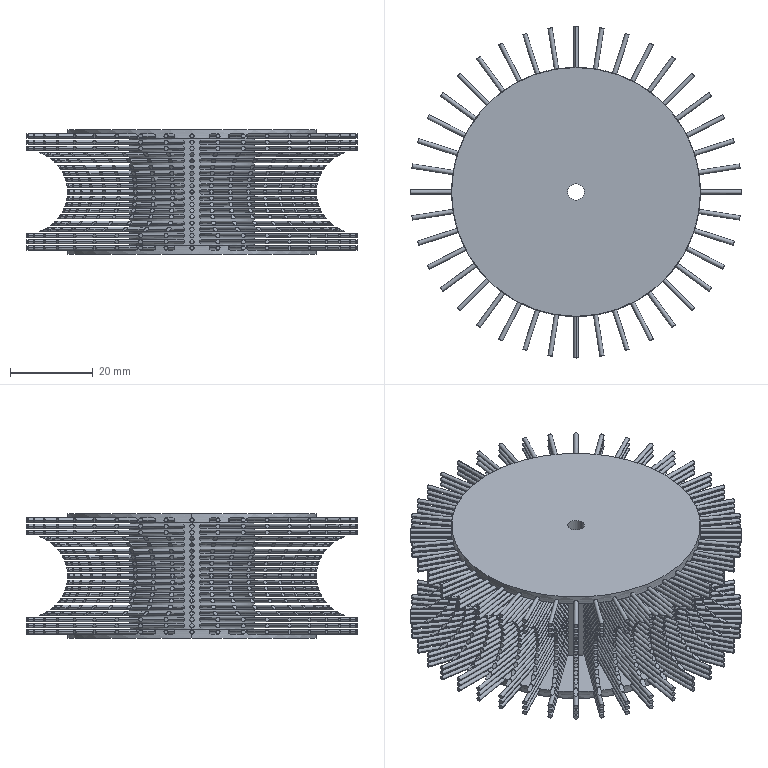Part | STEP file | Wheel brush | 1 solid | 2346 faces | box 80 x 80 x 30 mm | volume 40010 mm3 | cylinder 1528 | torus 574 | plane 244 | commonest cylinder face diameters 1 x1520 60 x4 4 x2 30 x2